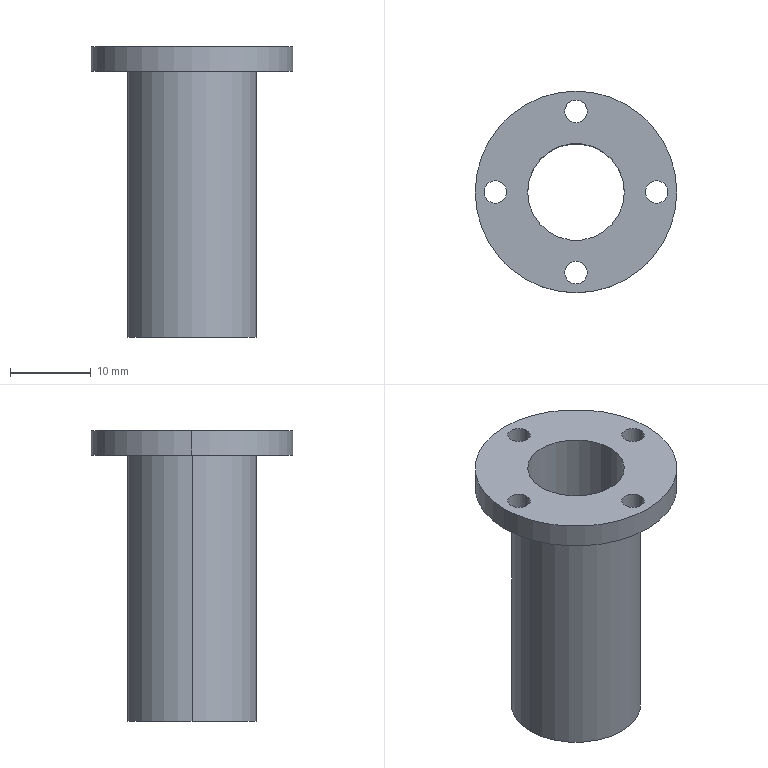Part | STEP file | Bushing | 1 solid | 17 faces | box 25 x 25 x 36 mm | volume 3962 mm3 | cylinder 14 | plane 3 | commonest cylinder face diameters 2.8 x8 12 x2 16 x2 25 x2
STEP:
#1=CARTESIAN_POINT('',(8.6,0.,33.));
#2=VERTEX_POINT('',#1);
#3=CARTESIAN_POINT('',(11.4,0.,33.));
#4=VERTEX_POINT('',#3);
#5=CARTESIAN_POINT('',(10.,0.,33.));
#6=DIRECTION('',(0.,0.,1.));
#7=DIRECTION('',(-1.,0.,0.));
#8=AXIS2_PLACEMENT_3D('',#5,#6,#7);
#9=CIRCLE('',#8,1.4);
#10=EDGE_CURVE('',#2,#4,#9,.T.);
#11=ORIENTED_EDGE('',*,*,#10,.F.);
#12=CARTESIAN_POINT('',(8.6,0.,36.));
#13=VERTEX_POINT('',#12);
#14=CARTESIAN_POINT('',(8.6,0.,33.));
#15=DIRECTION('',(0.,0.,1.));
#16=VECTOR('',#15,1000.);
#17=LINE('',#14,#16);
#18=EDGE_CURVE('',#2,#13,#17,.T.);
#19=ORIENTED_EDGE('',*,*,#18,.T.);
#20=CARTESIAN_POINT('',(11.4,0.,36.));
#21=VERTEX_POINT('',#20);
#22=CARTESIAN_POINT('',(10.,0.,36.));
#23=DIRECTION('',(0.,0.,1.));
#24=DIRECTION('',(-1.,0.,0.));
#25=AXIS2_PLACEMENT_3D('',#22,#23,#24);
#26=CIRCLE('',#25,1.4);
#27=EDGE_CURVE('',#13,#21,#26,.T.);
#28=ORIENTED_EDGE('',*,*,#27,.T.);
#29=CARTESIAN_POINT('',(11.4,0.,33.));
#30=DIRECTION('',(0.,0.,1.));
#31=VECTOR('',#30,1000.);
#32=LINE('',#29,#31);
#33=EDGE_CURVE('',#4,#21,#32,.T.);
#34=ORIENTED_EDGE('',*,*,#33,.F.);
#35=EDGE_LOOP('',(#11,#19,#28,#34));
#36=FACE_OUTER_BOUND('',#35,.T.);
#37=CARTESIAN_POINT('',(10.,0.,33.));
#38=DIRECTION('',(0.,0.,1.));
#39=DIRECTION('',(1.,0.,0.));
#40=AXIS2_PLACEMENT_3D('',#37,#38,#39);
#41=CYLINDRICAL_SURFACE('',#40,1.4);
#42=ADVANCED_FACE('',(#36),#41,.F.);
#43=CARTESIAN_POINT('',(-1.4,10.,33.));
#44=VERTEX_POINT('',#43);
#45=CARTESIAN_POINT('',(1.4,10.,33.));
#46=VERTEX_POINT('',#45);
#47=CARTESIAN_POINT('',(0.,10.,33.));
#48=DIRECTION('',(0.,0.,1.));
#49=DIRECTION('',(0.,-1.,0.));
#50=AXIS2_PLACEMENT_3D('',#47,#48,#49);
#51=CIRCLE('',#50,1.4);
#52=EDGE_CURVE('',#44,#46,#51,.T.);
#53=ORIENTED_EDGE('',*,*,#52,.F.);
#54=CARTESIAN_POINT('',(-1.4,10.,36.));
#55=VERTEX_POINT('',#54);
#56=CARTESIAN_POINT('',(-1.4,10.,33.));
#57=DIRECTION('',(0.,0.,1.));
#58=VECTOR('',#57,1000.);
#59=LINE('',#56,#58);
#60=EDGE_CURVE('',#44,#55,#59,.T.);
#61=ORIENTED_EDGE('',*,*,#60,.T.);
#62=CARTESIAN_POINT('',(1.4,10.,36.));
#63=VERTEX_POINT('',#62);
#64=CARTESIAN_POINT('',(0.,10.,36.));
#65=DIRECTION('',(0.,0.,1.));
#66=DIRECTION('',(0.,-1.,0.));
#67=AXIS2_PLACEMENT_3D('',#64,#65,#66);
#68=CIRCLE('',#67,1.4);
#69=EDGE_CURVE('',#55,#63,#68,.T.);
#70=ORIENTED_EDGE('',*,*,#69,.T.);
#71=CARTESIAN_POINT('',(1.4,10.,33.));
#72=DIRECTION('',(0.,0.,1.));
#73=VECTOR('',#72,1000.);
#74=LINE('',#71,#73);
#75=EDGE_CURVE('',#46,#63,#74,.T.);
#76=ORIENTED_EDGE('',*,*,#75,.F.);
#77=EDGE_LOOP('',(#53,#61,#70,#76));
#78=FACE_OUTER_BOUND('',#77,.T.);
#79=CARTESIAN_POINT('',(0.,10.,33.));
#80=DIRECTION('',(0.,0.,1.));
#81=DIRECTION('',(1.,0.,0.));
#82=AXIS2_PLACEMENT_3D('',#79,#80,#81);
#83=CYLINDRICAL_SURFACE('',#82,1.4);
#84=ADVANCED_FACE('',(#78),#83,.F.);
#85=CARTESIAN_POINT('',(-1.4,-10.,33.));
#86=VERTEX_POINT('',#85);
#87=CARTESIAN_POINT('',(1.4,-10.,33.));
#88=VERTEX_POINT('',#87);
#89=CARTESIAN_POINT('',(0.,-10.,33.));
#90=DIRECTION('',(0.,0.,1.));
#91=DIRECTION('',(0.,1.,0.));
#92=AXIS2_PLACEMENT_3D('',#89,#90,#91);
#93=CIRCLE('',#92,1.4);
#94=EDGE_CURVE('',#86,#88,#93,.T.);
#95=ORIENTED_EDGE('',*,*,#94,.F.);
#96=CARTESIAN_POINT('',(-1.4,-10.,36.));
#97=VERTEX_POINT('',#96);
#98=CARTESIAN_POINT('',(-1.4,-10.,33.));
#99=DIRECTION('',(0.,0.,1.));
#100=VECTOR('',#99,1000.);
#101=LINE('',#98,#100);
#102=EDGE_CURVE('',#86,#97,#101,.T.);
#103=ORIENTED_EDGE('',*,*,#102,.T.);
#104=CARTESIAN_POINT('',(1.4,-10.,36.));
#105=VERTEX_POINT('',#104);
#106=CARTESIAN_POINT('',(0.,-10.,36.));
#107=DIRECTION('',(0.,0.,1.));
#108=DIRECTION('',(0.,1.,0.));
#109=AXIS2_PLACEMENT_3D('',#106,#107,#108);
#110=CIRCLE('',#109,1.4);
#111=EDGE_CURVE('',#97,#105,#110,.T.);
#112=ORIENTED_EDGE('',*,*,#111,.T.);
#113=CARTESIAN_POINT('',(1.4,-10.,33.));
#114=DIRECTION('',(0.,0.,1.));
#115=VECTOR('',#114,1000.);
#116=LINE('',#113,#115);
#117=EDGE_CURVE('',#88,#105,#116,.T.);
#118=ORIENTED_EDGE('',*,*,#117,.F.);
#119=EDGE_LOOP('',(#95,#103,#112,#118));
#120=FACE_OUTER_BOUND('',#119,.T.);
#121=CARTESIAN_POINT('',(0.,-10.,33.));
#122=DIRECTION('',(0.,0.,1.));
#123=DIRECTION('',(1.,0.,0.));
#124=AXIS2_PLACEMENT_3D('',#121,#122,#123);
#125=CYLINDRICAL_SURFACE('',#124,1.4);
#126=ADVANCED_FACE('',(#120),#125,.F.);
#127=CARTESIAN_POINT('',(-11.4,0.,33.));
#128=VERTEX_POINT('',#127);
#129=CARTESIAN_POINT('',(-8.6,0.,33.));
#130=VERTEX_POINT('',#129);
#131=CARTESIAN_POINT('',(-10.,0.,33.));
#132=DIRECTION('',(0.,0.,1.));
#133=DIRECTION('',(1.,0.,0.));
#134=AXIS2_PLACEMENT_3D('',#131,#132,#133);
#135=CIRCLE('',#134,1.4);
#136=EDGE_CURVE('',#128,#130,#135,.T.);
#137=ORIENTED_EDGE('',*,*,#136,.F.);
#138=CARTESIAN_POINT('',(-11.4,0.,36.));
#139=VERTEX_POINT('',#138);
#140=CARTESIAN_POINT('',(-11.4,0.,33.));
#141=DIRECTION('',(0.,0.,1.));
#142=VECTOR('',#141,1000.);
#143=LINE('',#140,#142);
#144=EDGE_CURVE('',#128,#139,#143,.T.);
#145=ORIENTED_EDGE('',*,*,#144,.T.);
#146=CARTESIAN_POINT('',(-8.6,0.,36.));
#147=VERTEX_POINT('',#146);
#148=CARTESIAN_POINT('',(-10.,0.,36.));
#149=DIRECTION('',(0.,0.,1.));
#150=DIRECTION('',(1.,0.,0.));
#151=AXIS2_PLACEMENT_3D('',#148,#149,#150);
#152=CIRCLE('',#151,1.4);
#153=EDGE_CURVE('',#139,#147,#152,.T.);
#154=ORIENTED_EDGE('',*,*,#153,.T.);
#155=CARTESIAN_POINT('',(-8.6,0.,33.));
#156=DIRECTION('',(0.,0.,1.));
#157=VECTOR('',#156,1000.);
#158=LINE('',#155,#157);
#159=EDGE_CURVE('',#130,#147,#158,.T.);
#160=ORIENTED_EDGE('',*,*,#159,.F.);
#161=EDGE_LOOP('',(#137,#145,#154,#160));
#162=FACE_OUTER_BOUND('',#161,.T.);
#163=CARTESIAN_POINT('',(-10.,0.,33.));
#164=DIRECTION('',(0.,0.,1.));
#165=DIRECTION('',(1.,0.,0.));
#166=AXIS2_PLACEMENT_3D('',#163,#164,#165);
#167=CYLINDRICAL_SURFACE('',#166,1.4);
#168=ADVANCED_FACE('',(#162),#167,.F.);
#169=CARTESIAN_POINT('',(12.5,0.,33.));
#170=VERTEX_POINT('',#169);
#171=CARTESIAN_POINT('',(-12.5,0.,33.));
#172=VERTEX_POINT('',#171);
#173=CARTESIAN_POINT('',(0.,0.,33.));
#174=DIRECTION('',(0.,0.,1.));
#175=DIRECTION('',(1.,0.,0.));
#176=AXIS2_PLACEMENT_3D('',#173,#174,#175);
#177=CIRCLE('',#176,12.5);
#178=EDGE_CURVE('',#170,#172,#177,.T.);
#179=ORIENTED_EDGE('',*,*,#178,.T.);
#180=CARTESIAN_POINT('',(-12.5,0.,36.));
#181=VERTEX_POINT('',#180);
#182=CARTESIAN_POINT('',(-12.5,0.,33.));
#183=DIRECTION('',(0.,0.,1.));
#184=VECTOR('',#183,1000.);
#185=LINE('',#182,#184);
#186=EDGE_CURVE('',#172,#181,#185,.T.);
#187=ORIENTED_EDGE('',*,*,#186,.T.);
#188=CARTESIAN_POINT('',(12.5,0.,36.));
#189=VERTEX_POINT('',#188);
#190=CARTESIAN_POINT('',(0.,0.,36.));
#191=DIRECTION('',(0.,0.,1.));
#192=DIRECTION('',(1.,0.,0.));
#193=AXIS2_PLACEMENT_3D('',#190,#191,#192);
#194=CIRCLE('',#193,12.5);
#195=EDGE_CURVE('',#189,#181,#194,.T.);
#196=ORIENTED_EDGE('',*,*,#195,.F.);
#197=CARTESIAN_POINT('',(12.5,0.,33.));
#198=DIRECTION('',(0.,0.,1.));
#199=VECTOR('',#198,1000.);
#200=LINE('',#197,#199);
#201=EDGE_CURVE('',#170,#189,#200,.T.);
#202=ORIENTED_EDGE('',*,*,#201,.F.);
#203=EDGE_LOOP('',(#179,#187,#196,#202));
#204=FACE_OUTER_BOUND('',#203,.T.);
#205=CARTESIAN_POINT('',(0.,0.,33.));
#206=DIRECTION('',(0.,0.,1.));
#207=DIRECTION('',(1.,0.,0.));
#208=AXIS2_PLACEMENT_3D('',#205,#206,#207);
#209=CYLINDRICAL_SURFACE('',#208,12.5);
#210=ADVANCED_FACE('',(#204),#209,.T.);
#211=CARTESIAN_POINT('',(-6.,0.,36.));
#212=VERTEX_POINT('',#211);
#213=CARTESIAN_POINT('',(6.,0.,36.));
#214=VERTEX_POINT('',#213);
#215=CARTESIAN_POINT('',(0.,0.,36.));
#216=DIRECTION('',(0.,0.,1.));
#217=DIRECTION('',(1.,0.,0.));
#218=AXIS2_PLACEMENT_3D('',#215,#216,#217);
#219=CIRCLE('',#218,6.);
#220=EDGE_CURVE('',#212,#214,#219,.T.);
#221=ORIENTED_EDGE('',*,*,#220,.T.);
#222=CARTESIAN_POINT('',(6.,0.,0.));
#223=VERTEX_POINT('',#222);
#224=CARTESIAN_POINT('',(6.,0.,36.));
#225=DIRECTION('',(0.,0.,-1.));
#226=VECTOR('',#225,1000.);
#227=LINE('',#224,#226);
#228=EDGE_CURVE('',#214,#223,#227,.T.);
#229=ORIENTED_EDGE('',*,*,#228,.T.);
#230=CARTESIAN_POINT('',(-6.,0.,0.));
#231=VERTEX_POINT('',#230);
#232=CARTESIAN_POINT('',(0.,0.,0.));
#233=DIRECTION('',(0.,0.,1.));
#234=DIRECTION('',(1.,0.,0.));
#235=AXIS2_PLACEMENT_3D('',#232,#233,#234);
#236=CIRCLE('',#235,6.);
#237=EDGE_CURVE('',#231,#223,#236,.T.);
#238=ORIENTED_EDGE('',*,*,#237,.F.);
#239=CARTESIAN_POINT('',(-6.,0.,36.));
#240=DIRECTION('',(0.,0.,-1.));
#241=VECTOR('',#240,1000.);
#242=LINE('',#239,#241);
#243=EDGE_CURVE('',#212,#231,#242,.T.);
#244=ORIENTED_EDGE('',*,*,#243,.F.);
#245=EDGE_LOOP('',(#221,#229,#238,#244));
#246=FACE_OUTER_BOUND('',#245,.T.);
#247=CARTESIAN_POINT('',(0.,0.,36.));
#248=DIRECTION('',(0.,0.,-1.));
#249=DIRECTION('',(-1.,0.,0.));
#250=AXIS2_PLACEMENT_3D('',#247,#248,#249);
#251=CYLINDRICAL_SURFACE('',#250,6.);
#252=ADVANCED_FACE('',(#246),#251,.F.);
#253=CARTESIAN_POINT('',(8.,0.,33.));
#254=VERTEX_POINT('',#253);
#255=CARTESIAN_POINT('',(-8.,0.,33.));
#256=VERTEX_POINT('',#255);
#257=CARTESIAN_POINT('',(0.,0.,33.));
#258=DIRECTION('',(0.,0.,1.));
#259=DIRECTION('',(1.,0.,0.));
#260=AXIS2_PLACEMENT_3D('',#257,#258,#259);
#261=CIRCLE('',#260,8.);
#262=EDGE_CURVE('',#254,#256,#261,.T.);
#263=ORIENTED_EDGE('',*,*,#262,.F.);
#264=CARTESIAN_POINT('',(8.,0.,0.));
#265=VERTEX_POINT('',#264);
#266=CARTESIAN_POINT('',(8.,0.,36.));
#267=DIRECTION('',(0.,0.,-1.));
#268=VECTOR('',#267,1000.);
#269=LINE('',#266,#268);
#270=EDGE_CURVE('',#254,#265,#269,.T.);
#271=ORIENTED_EDGE('',*,*,#270,.T.);
#272=CARTESIAN_POINT('',(-8.,0.,0.));
#273=VERTEX_POINT('',#272);
#274=CARTESIAN_POINT('',(0.,0.,0.));
#275=DIRECTION('',(0.,0.,1.));
#276=DIRECTION('',(1.,0.,0.));
#277=AXIS2_PLACEMENT_3D('',#274,#275,#276);
#278=CIRCLE('',#277,8.);
#279=EDGE_CURVE('',#265,#273,#278,.T.);
#280=ORIENTED_EDGE('',*,*,#279,.T.);
#281=CARTESIAN_POINT('',(-8.,0.,36.));
#282=DIRECTION('',(0.,0.,-1.));
#283=VECTOR('',#282,1000.);
#284=LINE('',#281,#283);
#285=EDGE_CURVE('',#256,#273,#284,.T.);
#286=ORIENTED_EDGE('',*,*,#285,.F.);
#287=EDGE_LOOP('',(#263,#271,#280,#286));
#288=FACE_OUTER_BOUND('',#287,.T.);
#289=CARTESIAN_POINT('',(0.,0.,36.));
#290=DIRECTION('',(0.,0.,-1.));
#291=DIRECTION('',(-1.,0.,0.));
#292=AXIS2_PLACEMENT_3D('',#289,#290,#291);
#293=CYLINDRICAL_SURFACE('',#292,8.);
#294=ADVANCED_FACE('',(#288),#293,.T.);
#295=ORIENTED_EDGE('',*,*,#270,.F.);
#296=CARTESIAN_POINT('',(0.,0.,33.));
#297=DIRECTION('',(0.,0.,1.));
#298=DIRECTION('',(1.,0.,0.));
#299=AXIS2_PLACEMENT_3D('',#296,#297,#298);
#300=CIRCLE('',#299,8.);
#301=EDGE_CURVE('',#256,#254,#300,.T.);
#302=ORIENTED_EDGE('',*,*,#301,.F.);
#303=ORIENTED_EDGE('',*,*,#285,.T.);
#304=CARTESIAN_POINT('',(0.,0.,0.));
#305=DIRECTION('',(0.,0.,1.));
#306=DIRECTION('',(1.,0.,0.));
#307=AXIS2_PLACEMENT_3D('',#304,#305,#306);
#308=CIRCLE('',#307,8.);
#309=EDGE_CURVE('',#273,#265,#308,.T.);
#310=ORIENTED_EDGE('',*,*,#309,.T.);
#311=EDGE_LOOP('',(#295,#302,#303,#310));
#312=FACE_OUTER_BOUND('',#311,.T.);
#313=CARTESIAN_POINT('',(0.,0.,36.));
#314=DIRECTION('',(0.,0.,-1.));
#315=DIRECTION('',(-1.,0.,0.));
#316=AXIS2_PLACEMENT_3D('',#313,#314,#315);
#317=CYLINDRICAL_SURFACE('',#316,8.);
#318=ADVANCED_FACE('',(#312),#317,.T.);
#319=CARTESIAN_POINT('',(10.,0.,36.));
#320=DIRECTION('',(0.,0.,1.));
#321=DIRECTION('',(-1.,0.,0.));
#322=AXIS2_PLACEMENT_3D('',#319,#320,#321);
#323=CIRCLE('',#322,1.4);
#324=EDGE_CURVE('',#21,#13,#323,.T.);
#325=ORIENTED_EDGE('',*,*,#324,.F.);
#326=ORIENTED_EDGE('',*,*,#27,.F.);
#327=EDGE_LOOP('',(#325,#326));
#328=FACE_BOUND('',#327,.T.);
#329=CARTESIAN_POINT('',(0.,10.,36.));
#330=DIRECTION('',(0.,0.,1.));
#331=DIRECTION('',(0.,-1.,0.));
#332=AXIS2_PLACEMENT_3D('',#329,#330,#331);
#333=CIRCLE('',#332,1.4);
#334=EDGE_CURVE('',#63,#55,#333,.T.);
#335=ORIENTED_EDGE('',*,*,#334,.F.);
#336=ORIENTED_EDGE('',*,*,#69,.F.);
#337=EDGE_LOOP('',(#335,#336));
#338=FACE_BOUND('',#337,.T.);
#339=CARTESIAN_POINT('',(0.,-10.,36.));
#340=DIRECTION('',(0.,0.,1.));
#341=DIRECTION('',(0.,1.,0.));
#342=AXIS2_PLACEMENT_3D('',#339,#340,#341);
#343=CIRCLE('',#342,1.4);
#344=EDGE_CURVE('',#105,#97,#343,.T.);
#345=ORIENTED_EDGE('',*,*,#344,.F.);
#346=ORIENTED_EDGE('',*,*,#111,.F.);
#347=EDGE_LOOP('',(#345,#346));
#348=FACE_BOUND('',#347,.T.);
#349=CARTESIAN_POINT('',(-10.,0.,36.));
#350=DIRECTION('',(0.,0.,1.));
#351=DIRECTION('',(1.,0.,0.));
#352=AXIS2_PLACEMENT_3D('',#349,#350,#351);
#353=CIRCLE('',#352,1.4);
#354=EDGE_CURVE('',#147,#139,#353,.T.);
#355=ORIENTED_EDGE('',*,*,#354,.F.);
#356=ORIENTED_EDGE('',*,*,#153,.F.);
#357=EDGE_LOOP('',(#355,#356));
#358=FACE_BOUND('',#357,.T.);
#359=ORIENTED_EDGE('',*,*,#220,.F.);
#360=CARTESIAN_POINT('',(0.,0.,36.));
#361=DIRECTION('',(0.,0.,1.));
#362=DIRECTION('',(1.,0.,0.));
#363=AXIS2_PLACEMENT_3D('',#360,#361,#362);
#364=CIRCLE('',#363,6.);
#365=EDGE_CURVE('',#214,#212,#364,.T.);
#366=ORIENTED_EDGE('',*,*,#365,.F.);
#367=EDGE_LOOP('',(#359,#366));
#368=FACE_BOUND('',#367,.T.);
#369=ORIENTED_EDGE('',*,*,#195,.T.);
#370=CARTESIAN_POINT('',(0.,0.,36.));
#371=DIRECTION('',(0.,0.,1.));
#372=DIRECTION('',(1.,0.,0.));
#373=AXIS2_PLACEMENT_3D('',#370,#371,#372);
#374=CIRCLE('',#373,12.5);
#375=EDGE_CURVE('',#181,#189,#374,.T.);
#376=ORIENTED_EDGE('',*,*,#375,.T.);
#377=EDGE_LOOP('',(#369,#376));
#378=FACE_OUTER_BOUND('',#377,.T.);
#379=CARTESIAN_POINT('',(0.,0.,36.));
#380=DIRECTION('',(0.,0.,1.));
#381=DIRECTION('',(1.,0.,0.));
#382=AXIS2_PLACEMENT_3D('',#379,#380,#381);
#383=PLANE('',#382);
#384=ADVANCED_FACE('',(#328,#338,#348,#358,#368,#378),#383,.T.);
#385=ORIENTED_EDGE('',*,*,#309,.F.);
#386=ORIENTED_EDGE('',*,*,#279,.F.);
#387=EDGE_LOOP('',(#385,#386));
#388=FACE_OUTER_BOUND('',#387,.T.);
#389=ORIENTED_EDGE('',*,*,#237,.T.);
#390=CARTESIAN_POINT('',(0.,0.,0.));
#391=DIRECTION('',(0.,0.,1.));
#392=DIRECTION('',(1.,0.,0.));
#393=AXIS2_PLACEMENT_3D('',#390,#391,#392);
#394=CIRCLE('',#393,6.);
#395=EDGE_CURVE('',#223,#231,#394,.T.);
#396=ORIENTED_EDGE('',*,*,#395,.T.);
#397=EDGE_LOOP('',(#389,#396));
#398=FACE_BOUND('',#397,.T.);
#399=CARTESIAN_POINT('',(0.,0.,0.));
#400=DIRECTION('',(0.,0.,1.));
#401=DIRECTION('',(1.,0.,0.));
#402=AXIS2_PLACEMENT_3D('',#399,#400,#401);
#403=PLANE('',#402);
#404=ADVANCED_FACE('',(#388,#398),#403,.F.);
#405=ORIENTED_EDGE('',*,*,#228,.F.);
#406=ORIENTED_EDGE('',*,*,#365,.T.);
#407=ORIENTED_EDGE('',*,*,#243,.T.);
#408=ORIENTED_EDGE('',*,*,#395,.F.);
#409=EDGE_LOOP('',(#405,#406,#407,#408));
#410=FACE_OUTER_BOUND('',#409,.T.);
#411=CARTESIAN_POINT('',(0.,0.,36.));
#412=DIRECTION('',(0.,0.,-1.));
#413=DIRECTION('',(-1.,0.,0.));
#414=AXIS2_PLACEMENT_3D('',#411,#412,#413);
#415=CYLINDRICAL_SURFACE('',#414,6.);
#416=ADVANCED_FACE('',(#410),#415,.F.);
#417=ORIENTED_EDGE('',*,*,#186,.F.);
#418=CARTESIAN_POINT('',(0.,0.,33.));
#419=DIRECTION('',(0.,0.,1.));
#420=DIRECTION('',(1.,0.,0.));
#421=AXIS2_PLACEMENT_3D('',#418,#419,#420);
#422=CIRCLE('',#421,12.5);
#423=EDGE_CURVE('',#172,#170,#422,.T.);
#424=ORIENTED_EDGE('',*,*,#423,.T.);
#425=ORIENTED_EDGE('',*,*,#201,.T.);
#426=ORIENTED_EDGE('',*,*,#375,.F.);
#427=EDGE_LOOP('',(#417,#424,#425,#426));
#428=FACE_OUTER_BOUND('',#427,.T.);
#429=CARTESIAN_POINT('',(0.,0.,33.));
#430=DIRECTION('',(0.,0.,1.));
#431=DIRECTION('',(1.,0.,0.));
#432=AXIS2_PLACEMENT_3D('',#429,#430,#431);
#433=CYLINDRICAL_SURFACE('',#432,12.5);
#434=ADVANCED_FACE('',(#428),#433,.T.);
#435=CARTESIAN_POINT('',(10.,0.,33.));
#436=DIRECTION('',(0.,0.,1.));
#437=DIRECTION('',(-1.,0.,0.));
#438=AXIS2_PLACEMENT_3D('',#435,#436,#437);
#439=CIRCLE('',#438,1.4);
#440=EDGE_CURVE('',#4,#2,#439,.T.);
#441=ORIENTED_EDGE('',*,*,#440,.T.);
#442=ORIENTED_EDGE('',*,*,#10,.T.);
#443=EDGE_LOOP('',(#441,#442));
#444=FACE_BOUND('',#443,.T.);
#445=CARTESIAN_POINT('',(0.,10.,33.));
#446=DIRECTION('',(0.,0.,1.));
#447=DIRECTION('',(0.,-1.,0.));
#448=AXIS2_PLACEMENT_3D('',#445,#446,#447);
#449=CIRCLE('',#448,1.4);
#450=EDGE_CURVE('',#46,#44,#449,.T.);
#451=ORIENTED_EDGE('',*,*,#450,.T.);
#452=ORIENTED_EDGE('',*,*,#52,.T.);
#453=EDGE_LOOP('',(#451,#452));
#454=FACE_BOUND('',#453,.T.);
#455=CARTESIAN_POINT('',(0.,-10.,33.));
#456=DIRECTION('',(0.,0.,1.));
#457=DIRECTION('',(0.,1.,0.));
#458=AXIS2_PLACEMENT_3D('',#455,#456,#457);
#459=CIRCLE('',#458,1.4);
#460=EDGE_CURVE('',#88,#86,#459,.T.);
#461=ORIENTED_EDGE('',*,*,#460,.T.);
#462=ORIENTED_EDGE('',*,*,#94,.T.);
#463=EDGE_LOOP('',(#461,#462));
#464=FACE_BOUND('',#463,.T.);
#465=CARTESIAN_POINT('',(-10.,0.,33.));
#466=DIRECTION('',(0.,0.,1.));
#467=DIRECTION('',(1.,0.,0.));
#468=AXIS2_PLACEMENT_3D('',#465,#466,#467);
#469=CIRCLE('',#468,1.4);
#470=EDGE_CURVE('',#130,#128,#469,.T.);
#471=ORIENTED_EDGE('',*,*,#470,.T.);
#472=ORIENTED_EDGE('',*,*,#136,.T.);
#473=EDGE_LOOP('',(#471,#472));
#474=FACE_BOUND('',#473,.T.);
#475=ORIENTED_EDGE('',*,*,#301,.T.);
#476=ORIENTED_EDGE('',*,*,#262,.T.);
#477=EDGE_LOOP('',(#475,#476));
#478=FACE_BOUND('',#477,.T.);
#479=ORIENTED_EDGE('',*,*,#178,.F.);
#480=ORIENTED_EDGE('',*,*,#423,.F.);
#481=EDGE_LOOP('',(#479,#480));
#482=FACE_OUTER_BOUND('',#481,.T.);
#483=CARTESIAN_POINT('',(0.,0.,33.));
#484=DIRECTION('',(0.,0.,1.));
#485=DIRECTION('',(1.,0.,0.));
#486=AXIS2_PLACEMENT_3D('',#483,#484,#485);
#487=PLANE('',#486);
#488=ADVANCED_FACE('',(#444,#454,#464,#474,#478,#482),#487,.F.);
#489=ORIENTED_EDGE('',*,*,#144,.F.);
#490=ORIENTED_EDGE('',*,*,#470,.F.);
#491=ORIENTED_EDGE('',*,*,#159,.T.);
#492=ORIENTED_EDGE('',*,*,#354,.T.);
#493=EDGE_LOOP('',(#489,#490,#491,#492));
#494=FACE_OUTER_BOUND('',#493,.T.);
#495=CARTESIAN_POINT('',(-10.,0.,33.));
#496=DIRECTION('',(0.,0.,1.));
#497=DIRECTION('',(1.,0.,0.));
#498=AXIS2_PLACEMENT_3D('',#495,#496,#497);
#499=CYLINDRICAL_SURFACE('',#498,1.4);
#500=ADVANCED_FACE('',(#494),#499,.F.);
#501=ORIENTED_EDGE('',*,*,#102,.F.);
#502=ORIENTED_EDGE('',*,*,#460,.F.);
#503=ORIENTED_EDGE('',*,*,#117,.T.);
#504=ORIENTED_EDGE('',*,*,#344,.T.);
#505=EDGE_LOOP('',(#501,#502,#503,#504));
#506=FACE_OUTER_BOUND('',#505,.T.);
#507=CARTESIAN_POINT('',(0.,-10.,33.));
#508=DIRECTION('',(0.,0.,1.));
#509=DIRECTION('',(1.,0.,0.));
#510=AXIS2_PLACEMENT_3D('',#507,#508,#509);
#511=CYLINDRICAL_SURFACE('',#510,1.4);
#512=ADVANCED_FACE('',(#506),#511,.F.);
#513=ORIENTED_EDGE('',*,*,#60,.F.);
#514=ORIENTED_EDGE('',*,*,#450,.F.);
#515=ORIENTED_EDGE('',*,*,#75,.T.);
#516=ORIENTED_EDGE('',*,*,#334,.T.);
#517=EDGE_LOOP('',(#513,#514,#515,#516));
#518=FACE_OUTER_BOUND('',#517,.T.);
#519=CARTESIAN_POINT('',(0.,10.,33.));
#520=DIRECTION('',(0.,0.,1.));
#521=DIRECTION('',(1.,0.,0.));
#522=AXIS2_PLACEMENT_3D('',#519,#520,#521);
#523=CYLINDRICAL_SURFACE('',#522,1.4);
#524=ADVANCED_FACE('',(#518),#523,.F.);
#525=ORIENTED_EDGE('',*,*,#18,.F.);
#526=ORIENTED_EDGE('',*,*,#440,.F.);
#527=ORIENTED_EDGE('',*,*,#33,.T.);
#528=ORIENTED_EDGE('',*,*,#324,.T.);
#529=EDGE_LOOP('',(#525,#526,#527,#528));
#530=FACE_OUTER_BOUND('',#529,.T.);
#531=CARTESIAN_POINT('',(10.,0.,33.));
#532=DIRECTION('',(0.,0.,1.));
#533=DIRECTION('',(1.,0.,0.));
#534=AXIS2_PLACEMENT_3D('',#531,#532,#533);
#535=CYLINDRICAL_SURFACE('',#534,1.4);
#536=ADVANCED_FACE('',(#530),#535,.F.);
#537=CLOSED_SHELL('',(#42,#84,#126,#168,#210,#252,#294,#318,#384,#404,#416,#434,#488,#500,#512,#524,#536));
#538=MANIFOLD_SOLID_BREP('',#537);
#539=CARTESIAN_POINT('',(0.,0.,0.));
#540=DIRECTION('',(0.,0.,1.));
#541=DIRECTION('',(1.,0.,0.));
#542=AXIS2_PLACEMENT_3D('',#539,#540,#541);
#543=(LENGTH_UNIT()NAMED_UNIT(*)SI_UNIT(.MILLI.,.METRE.));
#544=UNCERTAINTY_MEASURE_WITH_UNIT(LENGTH_MEASURE(0.00001),#543,'','');
#545=(NAMED_UNIT(*)PLANE_ANGLE_UNIT()SI_UNIT($,.RADIAN.));
#546=(NAMED_UNIT(*)SI_UNIT($,.STERADIAN.)SOLID_ANGLE_UNIT());
#547=(GEOMETRIC_REPRESENTATION_CONTEXT(3)GLOBAL_UNCERTAINTY_ASSIGNED_CONTEXT((#544))GLOBAL_UNIT_ASSIGNED_CONTEXT((#543,#545,#546))REPRESENTATION_CONTEXT('',''));
#548=ADVANCED_BREP_SHAPE_REPRESENTATION('',(#538,#542),#547);